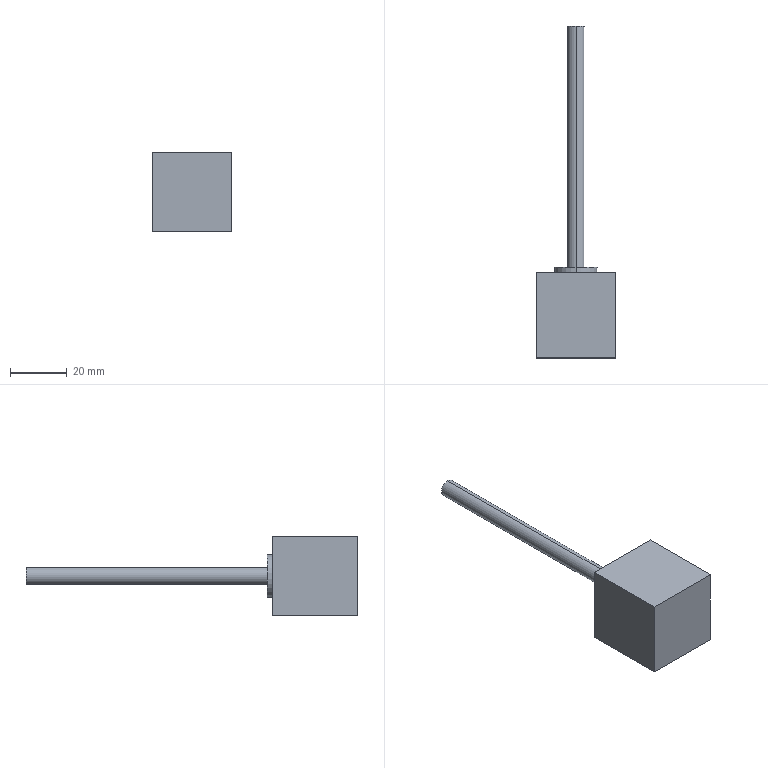Part | SolidWorks | features ICE 3, Extrusion 1, HoleWzd 1 | 1 solid | 28 faces | box 28 x 117 x 28 mm | volume 26125 mm3 | cylinder 12 | cone 8 | plane 8 | commonest cylinder face diameters 2.5 x8 6 x2 15 x2
STEP:
#1=CARTESIAN_POINT('',(-11.5,22.5,10.25));
#2=VERTEX_POINT('',#1);
#3=CARTESIAN_POINT('',(-11.5,22.5,12.75));
#4=VERTEX_POINT('',#3);
#5=CARTESIAN_POINT('',(-11.5,22.5,11.5));
#6=DIRECTION('',(0.,1.,0.));
#7=DIRECTION('',(0.,0.,1.));
#8=AXIS2_PLACEMENT_3D('',#5,#6,#7);
#9=CIRCLE('',#8,1.25);
#10=EDGE_CURVE('',#2,#4,#9,.T.);
#11=ORIENTED_EDGE('',*,*,#10,.F.);
#12=CARTESIAN_POINT('',(-11.5,30.,10.25));
#13=VERTEX_POINT('',#12);
#14=CARTESIAN_POINT('',(-11.5,30.,10.25));
#15=DIRECTION('',(0.,1.,0.));
#16=VECTOR('',#15,1000.);
#17=LINE('',#14,#16);
#18=EDGE_CURVE('',#2,#13,#17,.T.);
#19=ORIENTED_EDGE('',*,*,#18,.T.);
#20=CARTESIAN_POINT('',(-11.5,30.,12.75));
#21=VERTEX_POINT('',#20);
#22=CARTESIAN_POINT('',(-11.5,30.,11.5));
#23=DIRECTION('',(0.,1.,0.));
#24=DIRECTION('',(0.,0.,1.));
#25=AXIS2_PLACEMENT_3D('',#22,#23,#24);
#26=CIRCLE('',#25,1.25);
#27=EDGE_CURVE('',#13,#21,#26,.T.);
#28=ORIENTED_EDGE('',*,*,#27,.T.);
#29=CARTESIAN_POINT('',(-11.5,30.,12.75));
#30=DIRECTION('',(0.,1.,0.));
#31=VECTOR('',#30,1000.);
#32=LINE('',#29,#31);
#33=EDGE_CURVE('',#4,#21,#32,.T.);
#34=ORIENTED_EDGE('',*,*,#33,.F.);
#35=EDGE_LOOP('',(#11,#19,#28,#34));
#36=FACE_OUTER_BOUND('',#35,.T.);
#37=CARTESIAN_POINT('',(-11.5,30.,11.5));
#38=DIRECTION('',(0.,1.,0.));
#39=DIRECTION('',(0.,0.,1.));
#40=AXIS2_PLACEMENT_3D('',#37,#38,#39);
#41=CYLINDRICAL_SURFACE('',#40,1.25);
#42=ADVANCED_FACE('',(#36),#41,.F.);
#43=CARTESIAN_POINT('',(-11.5,21.749,11.5));
#44=VERTEX_POINT('',#43);
#45=CARTESIAN_POINT('',(-11.5,22.5,12.75));
#46=DIRECTION('',(0.,0.515,0.8572));
#47=VECTOR('',#46,1000.);
#48=LINE('',#45,#47);
#49=EDGE_CURVE('',#44,#4,#48,.T.);
#50=ORIENTED_EDGE('',*,*,#49,.F.);
#51=CARTESIAN_POINT('',(-11.5,22.5,10.25));
#52=DIRECTION('',(0.,0.515,-0.8572));
#53=VECTOR('',#52,1000.);
#54=LINE('',#51,#53);
#55=EDGE_CURVE('',#44,#2,#54,.T.);
#56=ORIENTED_EDGE('',*,*,#55,.T.);
#57=ORIENTED_EDGE('',*,*,#10,.T.);
#58=EDGE_LOOP('',(#50,#56,#57));
#59=FACE_OUTER_BOUND('',#58,.T.);
#60=CARTESIAN_POINT('',(-11.5,22.5,11.5));
#61=DIRECTION('',(0.,1.,0.));
#62=DIRECTION('',(0.,0.,1.));
#63=AXIS2_PLACEMENT_3D('',#60,#61,#62);
#64=CONICAL_SURFACE('',#63,1.25,1.03);
#65=ADVANCED_FACE('',(#59),#64,.F.);
#66=CARTESIAN_POINT('',(11.5,22.5,10.25));
#67=VERTEX_POINT('',#66);
#68=CARTESIAN_POINT('',(11.5,22.5,12.75));
#69=VERTEX_POINT('',#68);
#70=CARTESIAN_POINT('',(11.5,22.5,11.5));
#71=DIRECTION('',(0.,1.,0.));
#72=DIRECTION('',(0.,0.,1.));
#73=AXIS2_PLACEMENT_3D('',#70,#71,#72);
#74=CIRCLE('',#73,1.25);
#75=EDGE_CURVE('',#67,#69,#74,.T.);
#76=ORIENTED_EDGE('',*,*,#75,.F.);
#77=CARTESIAN_POINT('',(11.5,30.,10.25));
#78=VERTEX_POINT('',#77);
#79=CARTESIAN_POINT('',(11.5,30.,10.25));
#80=DIRECTION('',(0.,1.,0.));
#81=VECTOR('',#80,1000.);
#82=LINE('',#79,#81);
#83=EDGE_CURVE('',#67,#78,#82,.T.);
#84=ORIENTED_EDGE('',*,*,#83,.T.);
#85=CARTESIAN_POINT('',(11.5,30.,12.75));
#86=VERTEX_POINT('',#85);
#87=CARTESIAN_POINT('',(11.5,30.,11.5));
#88=DIRECTION('',(0.,1.,0.));
#89=DIRECTION('',(0.,0.,1.));
#90=AXIS2_PLACEMENT_3D('',#87,#88,#89);
#91=CIRCLE('',#90,1.25);
#92=EDGE_CURVE('',#78,#86,#91,.T.);
#93=ORIENTED_EDGE('',*,*,#92,.T.);
#94=CARTESIAN_POINT('',(11.5,30.,12.75));
#95=DIRECTION('',(0.,1.,0.));
#96=VECTOR('',#95,1000.);
#97=LINE('',#94,#96);
#98=EDGE_CURVE('',#69,#86,#97,.T.);
#99=ORIENTED_EDGE('',*,*,#98,.F.);
#100=EDGE_LOOP('',(#76,#84,#93,#99));
#101=FACE_OUTER_BOUND('',#100,.T.);
#102=CARTESIAN_POINT('',(11.5,30.,11.5));
#103=DIRECTION('',(0.,1.,0.));
#104=DIRECTION('',(0.,0.,1.));
#105=AXIS2_PLACEMENT_3D('',#102,#103,#104);
#106=CYLINDRICAL_SURFACE('',#105,1.25);
#107=ADVANCED_FACE('',(#101),#106,.F.);
#108=CARTESIAN_POINT('',(11.5,21.749,11.5));
#109=VERTEX_POINT('',#108);
#110=CARTESIAN_POINT('',(11.5,22.5,12.75));
#111=DIRECTION('',(0.,0.515,0.8572));
#112=VECTOR('',#111,1000.);
#113=LINE('',#110,#112);
#114=EDGE_CURVE('',#109,#69,#113,.T.);
#115=ORIENTED_EDGE('',*,*,#114,.F.);
#116=CARTESIAN_POINT('',(11.5,22.5,10.25));
#117=DIRECTION('',(0.,0.515,-0.8572));
#118=VECTOR('',#117,1000.);
#119=LINE('',#116,#118);
#120=EDGE_CURVE('',#109,#67,#119,.T.);
#121=ORIENTED_EDGE('',*,*,#120,.T.);
#122=ORIENTED_EDGE('',*,*,#75,.T.);
#123=EDGE_LOOP('',(#115,#121,#122));
#124=FACE_OUTER_BOUND('',#123,.T.);
#125=CARTESIAN_POINT('',(11.5,22.5,11.5));
#126=DIRECTION('',(0.,1.,0.));
#127=DIRECTION('',(0.,0.,1.));
#128=AXIS2_PLACEMENT_3D('',#125,#126,#127);
#129=CONICAL_SURFACE('',#128,1.25,1.03);
#130=ADVANCED_FACE('',(#124),#129,.F.);
#131=CARTESIAN_POINT('',(-11.5,22.5,-12.75));
#132=VERTEX_POINT('',#131);
#133=CARTESIAN_POINT('',(-11.5,22.5,-10.25));
#134=VERTEX_POINT('',#133);
#135=CARTESIAN_POINT('',(-11.5,22.5,-11.5));
#136=DIRECTION('',(0.,1.,0.));
#137=DIRECTION('',(0.,0.,1.));
#138=AXIS2_PLACEMENT_3D('',#135,#136,#137);
#139=CIRCLE('',#138,1.25);
#140=EDGE_CURVE('',#132,#134,#139,.T.);
#141=ORIENTED_EDGE('',*,*,#140,.F.);
#142=CARTESIAN_POINT('',(-11.5,30.,-12.75));
#143=VERTEX_POINT('',#142);
#144=CARTESIAN_POINT('',(-11.5,30.,-12.75));
#145=DIRECTION('',(0.,1.,0.));
#146=VECTOR('',#145,1000.);
#147=LINE('',#144,#146);
#148=EDGE_CURVE('',#132,#143,#147,.T.);
#149=ORIENTED_EDGE('',*,*,#148,.T.);
#150=CARTESIAN_POINT('',(-11.5,30.,-10.25));
#151=VERTEX_POINT('',#150);
#152=CARTESIAN_POINT('',(-11.5,30.,-11.5));
#153=DIRECTION('',(0.,1.,0.));
#154=DIRECTION('',(0.,0.,1.));
#155=AXIS2_PLACEMENT_3D('',#152,#153,#154);
#156=CIRCLE('',#155,1.25);
#157=EDGE_CURVE('',#143,#151,#156,.T.);
#158=ORIENTED_EDGE('',*,*,#157,.T.);
#159=CARTESIAN_POINT('',(-11.5,30.,-10.25));
#160=DIRECTION('',(0.,1.,0.));
#161=VECTOR('',#160,1000.);
#162=LINE('',#159,#161);
#163=EDGE_CURVE('',#134,#151,#162,.T.);
#164=ORIENTED_EDGE('',*,*,#163,.F.);
#165=EDGE_LOOP('',(#141,#149,#158,#164));
#166=FACE_OUTER_BOUND('',#165,.T.);
#167=CARTESIAN_POINT('',(-11.5,30.,-11.5));
#168=DIRECTION('',(0.,1.,0.));
#169=DIRECTION('',(0.,0.,1.));
#170=AXIS2_PLACEMENT_3D('',#167,#168,#169);
#171=CYLINDRICAL_SURFACE('',#170,1.25);
#172=ADVANCED_FACE('',(#166),#171,.F.);
#173=CARTESIAN_POINT('',(-11.5,21.749,-11.5));
#174=VERTEX_POINT('',#173);
#175=CARTESIAN_POINT('',(-11.5,22.5,-10.25));
#176=DIRECTION('',(0.,0.515,0.8572));
#177=VECTOR('',#176,1000.);
#178=LINE('',#175,#177);
#179=EDGE_CURVE('',#174,#134,#178,.T.);
#180=ORIENTED_EDGE('',*,*,#179,.F.);
#181=CARTESIAN_POINT('',(-11.5,22.5,-12.75));
#182=DIRECTION('',(0.,0.515,-0.8572));
#183=VECTOR('',#182,1000.);
#184=LINE('',#181,#183);
#185=EDGE_CURVE('',#174,#132,#184,.T.);
#186=ORIENTED_EDGE('',*,*,#185,.T.);
#187=ORIENTED_EDGE('',*,*,#140,.T.);
#188=EDGE_LOOP('',(#180,#186,#187));
#189=FACE_OUTER_BOUND('',#188,.T.);
#190=CARTESIAN_POINT('',(-11.5,22.5,-11.5));
#191=DIRECTION('',(0.,1.,0.));
#192=DIRECTION('',(0.,0.,1.));
#193=AXIS2_PLACEMENT_3D('',#190,#191,#192);
#194=CONICAL_SURFACE('',#193,1.25,1.03);
#195=ADVANCED_FACE('',(#189),#194,.F.);
#196=CARTESIAN_POINT('',(11.5,22.5,-12.75));
#197=VERTEX_POINT('',#196);
#198=CARTESIAN_POINT('',(11.5,22.5,-10.25));
#199=VERTEX_POINT('',#198);
#200=CARTESIAN_POINT('',(11.5,22.5,-11.5));
#201=DIRECTION('',(0.,1.,0.));
#202=DIRECTION('',(0.,0.,1.));
#203=AXIS2_PLACEMENT_3D('',#200,#201,#202);
#204=CIRCLE('',#203,1.25);
#205=EDGE_CURVE('',#197,#199,#204,.T.);
#206=ORIENTED_EDGE('',*,*,#205,.F.);
#207=CARTESIAN_POINT('',(11.5,30.,-12.75));
#208=VERTEX_POINT('',#207);
#209=CARTESIAN_POINT('',(11.5,30.,-12.75));
#210=DIRECTION('',(0.,1.,0.));
#211=VECTOR('',#210,1000.);
#212=LINE('',#209,#211);
#213=EDGE_CURVE('',#197,#208,#212,.T.);
#214=ORIENTED_EDGE('',*,*,#213,.T.);
#215=CARTESIAN_POINT('',(11.5,30.,-10.25));
#216=VERTEX_POINT('',#215);
#217=CARTESIAN_POINT('',(11.5,30.,-11.5));
#218=DIRECTION('',(0.,1.,0.));
#219=DIRECTION('',(0.,0.,1.));
#220=AXIS2_PLACEMENT_3D('',#217,#218,#219);
#221=CIRCLE('',#220,1.25);
#222=EDGE_CURVE('',#208,#216,#221,.T.);
#223=ORIENTED_EDGE('',*,*,#222,.T.);
#224=CARTESIAN_POINT('',(11.5,30.,-10.25));
#225=DIRECTION('',(0.,1.,0.));
#226=VECTOR('',#225,1000.);
#227=LINE('',#224,#226);
#228=EDGE_CURVE('',#199,#216,#227,.T.);
#229=ORIENTED_EDGE('',*,*,#228,.F.);
#230=EDGE_LOOP('',(#206,#214,#223,#229));
#231=FACE_OUTER_BOUND('',#230,.T.);
#232=CARTESIAN_POINT('',(11.5,30.,-11.5));
#233=DIRECTION('',(0.,1.,0.));
#234=DIRECTION('',(0.,0.,1.));
#235=AXIS2_PLACEMENT_3D('',#232,#233,#234);
#236=CYLINDRICAL_SURFACE('',#235,1.25);
#237=ADVANCED_FACE('',(#231),#236,.F.);
#238=CARTESIAN_POINT('',(11.5,21.749,-11.5));
#239=VERTEX_POINT('',#238);
#240=CARTESIAN_POINT('',(11.5,22.5,-10.25));
#241=DIRECTION('',(0.,0.515,0.8572));
#242=VECTOR('',#241,1000.);
#243=LINE('',#240,#242);
#244=EDGE_CURVE('',#239,#199,#243,.T.);
#245=ORIENTED_EDGE('',*,*,#244,.F.);
#246=CARTESIAN_POINT('',(11.5,22.5,-12.75));
#247=DIRECTION('',(0.,0.515,-0.8572));
#248=VECTOR('',#247,1000.);
#249=LINE('',#246,#248);
#250=EDGE_CURVE('',#239,#197,#249,.T.);
#251=ORIENTED_EDGE('',*,*,#250,.T.);
#252=ORIENTED_EDGE('',*,*,#205,.T.);
#253=EDGE_LOOP('',(#245,#251,#252));
#254=FACE_OUTER_BOUND('',#253,.T.);
#255=CARTESIAN_POINT('',(11.5,22.5,-11.5));
#256=DIRECTION('',(0.,1.,0.));
#257=DIRECTION('',(0.,0.,1.));
#258=AXIS2_PLACEMENT_3D('',#255,#256,#257);
#259=CONICAL_SURFACE('',#258,1.25,1.03);
#260=ADVANCED_FACE('',(#254),#259,.F.);
#261=CARTESIAN_POINT('',(0.,117.,3.));
#262=VERTEX_POINT('',#261);
#263=CARTESIAN_POINT('',(0.,117.,-3.));
#264=VERTEX_POINT('',#263);
#265=CARTESIAN_POINT('',(0.,117.,0.));
#266=DIRECTION('',(0.,1.,0.));
#267=DIRECTION('',(0.,0.,1.));
#268=AXIS2_PLACEMENT_3D('',#265,#266,#267);
#269=CIRCLE('',#268,3.);
#270=EDGE_CURVE('',#262,#264,#269,.T.);
#271=ORIENTED_EDGE('',*,*,#270,.F.);
#272=CARTESIAN_POINT('',(0.,32.,3.));
#273=VERTEX_POINT('',#272);
#274=CARTESIAN_POINT('',(0.,117.,3.));
#275=DIRECTION('',(0.,-1.,0.));
#276=VECTOR('',#275,1000.);
#277=LINE('',#274,#276);
#278=EDGE_CURVE('',#262,#273,#277,.T.);
#279=ORIENTED_EDGE('',*,*,#278,.T.);
#280=CARTESIAN_POINT('',(0.,32.,-3.));
#281=VERTEX_POINT('',#280);
#282=CARTESIAN_POINT('',(0.,32.,0.));
#283=DIRECTION('',(0.,1.,0.));
#284=DIRECTION('',(0.,0.,1.));
#285=AXIS2_PLACEMENT_3D('',#282,#283,#284);
#286=CIRCLE('',#285,3.);
#287=EDGE_CURVE('',#273,#281,#286,.T.);
#288=ORIENTED_EDGE('',*,*,#287,.T.);
#289=CARTESIAN_POINT('',(0.,117.,-3.));
#290=DIRECTION('',(0.,-1.,0.));
#291=VECTOR('',#290,1000.);
#292=LINE('',#289,#291);
#293=EDGE_CURVE('',#264,#281,#292,.T.);
#294=ORIENTED_EDGE('',*,*,#293,.F.);
#295=EDGE_LOOP('',(#271,#279,#288,#294));
#296=FACE_OUTER_BOUND('',#295,.T.);
#297=CARTESIAN_POINT('',(0.,117.,0.));
#298=DIRECTION('',(0.,-1.,0.));
#299=DIRECTION('',(0.,0.,-1.));
#300=AXIS2_PLACEMENT_3D('',#297,#298,#299);
#301=CYLINDRICAL_SURFACE('',#300,3.);
#302=ADVANCED_FACE('',(#296),#301,.T.);
#303=CARTESIAN_POINT('',(0.,32.,7.5));
#304=VERTEX_POINT('',#303);
#305=CARTESIAN_POINT('',(0.,32.,-7.5));
#306=VERTEX_POINT('',#305);
#307=CARTESIAN_POINT('',(0.,32.,0.));
#308=DIRECTION('',(0.,1.,0.));
#309=DIRECTION('',(0.,0.,1.));
#310=AXIS2_PLACEMENT_3D('',#307,#308,#309);
#311=CIRCLE('',#310,7.5);
#312=EDGE_CURVE('',#304,#306,#311,.T.);
#313=ORIENTED_EDGE('',*,*,#312,.F.);
#314=CARTESIAN_POINT('',(0.,30.,7.5));
#315=VERTEX_POINT('',#314);
#316=CARTESIAN_POINT('',(0.,32.,7.5));
#317=DIRECTION('',(0.,-1.,0.));
#318=VECTOR('',#317,1000.);
#319=LINE('',#316,#318);
#320=EDGE_CURVE('',#304,#315,#319,.T.);
#321=ORIENTED_EDGE('',*,*,#320,.T.);
#322=CARTESIAN_POINT('',(0.,30.,-7.5));
#323=VERTEX_POINT('',#322);
#324=CARTESIAN_POINT('',(0.,30.,0.));
#325=DIRECTION('',(0.,1.,0.));
#326=DIRECTION('',(0.,0.,1.));
#327=AXIS2_PLACEMENT_3D('',#324,#325,#326);
#328=CIRCLE('',#327,7.5);
#329=EDGE_CURVE('',#315,#323,#328,.T.);
#330=ORIENTED_EDGE('',*,*,#329,.T.);
#331=CARTESIAN_POINT('',(0.,32.,-7.5));
#332=DIRECTION('',(0.,-1.,0.));
#333=VECTOR('',#332,1000.);
#334=LINE('',#331,#333);
#335=EDGE_CURVE('',#306,#323,#334,.T.);
#336=ORIENTED_EDGE('',*,*,#335,.F.);
#337=EDGE_LOOP('',(#313,#321,#330,#336));
#338=FACE_OUTER_BOUND('',#337,.T.);
#339=CARTESIAN_POINT('',(0.,32.,0.));
#340=DIRECTION('',(0.,-1.,0.));
#341=DIRECTION('',(0.,0.,-1.));
#342=AXIS2_PLACEMENT_3D('',#339,#340,#341);
#343=CYLINDRICAL_SURFACE('',#342,7.5);
#344=ADVANCED_FACE('',(#338),#343,.T.);
#345=CARTESIAN_POINT('',(14.,0.,14.));
#346=VERTEX_POINT('',#345);
#347=CARTESIAN_POINT('',(14.,0.,-14.));
#348=VERTEX_POINT('',#347);
#349=CARTESIAN_POINT('',(14.,0.,-14.));
#350=DIRECTION('',(0.,0.,-1.));
#351=VECTOR('',#350,1000.);
#352=LINE('',#349,#351);
#353=EDGE_CURVE('',#346,#348,#352,.T.);
#354=ORIENTED_EDGE('',*,*,#353,.T.);
#355=CARTESIAN_POINT('',(14.,30.,-14.));
#356=VERTEX_POINT('',#355);
#357=CARTESIAN_POINT('',(14.,30.,-14.));
#358=DIRECTION('',(0.,-1.,0.));
#359=VECTOR('',#358,1000.);
#360=LINE('',#357,#359);
#361=EDGE_CURVE('',#356,#348,#360,.T.);
#362=ORIENTED_EDGE('',*,*,#361,.F.);
#363=CARTESIAN_POINT('',(14.,30.,14.));
#364=VERTEX_POINT('',#363);
#365=CARTESIAN_POINT('',(14.,30.,-14.));
#366=DIRECTION('',(0.,0.,-1.));
#367=VECTOR('',#366,1000.);
#368=LINE('',#365,#367);
#369=EDGE_CURVE('',#364,#356,#368,.T.);
#370=ORIENTED_EDGE('',*,*,#369,.F.);
#371=CARTESIAN_POINT('',(14.,30.,14.));
#372=DIRECTION('',(0.,-1.,0.));
#373=VECTOR('',#372,1000.);
#374=LINE('',#371,#373);
#375=EDGE_CURVE('',#364,#346,#374,.T.);
#376=ORIENTED_EDGE('',*,*,#375,.T.);
#377=EDGE_LOOP('',(#354,#362,#370,#376));
#378=FACE_OUTER_BOUND('',#377,.T.);
#379=CARTESIAN_POINT('',(14.,30.,-14.));
#380=DIRECTION('',(-1.,0.,0.));
#381=DIRECTION('',(0.,0.,1.));
#382=AXIS2_PLACEMENT_3D('',#379,#380,#381);
#383=PLANE('',#382);
#384=ADVANCED_FACE('',(#378),#383,.F.);
#385=CARTESIAN_POINT('',(-14.,0.,-14.));
#386=VERTEX_POINT('',#385);
#387=CARTESIAN_POINT('',(-14.,0.,-14.));
#388=DIRECTION('',(-1.,0.,0.));
#389=VECTOR('',#388,1000.);
#390=LINE('',#387,#389);
#391=EDGE_CURVE('',#348,#386,#390,.T.);
#392=ORIENTED_EDGE('',*,*,#391,.T.);
#393=CARTESIAN_POINT('',(-14.,30.,-14.));
#394=VERTEX_POINT('',#393);
#395=CARTESIAN_POINT('',(-14.,30.,-14.));
#396=DIRECTION('',(0.,-1.,0.));
#397=VECTOR('',#396,1000.);
#398=LINE('',#395,#397);
#399=EDGE_CURVE('',#394,#386,#398,.T.);
#400=ORIENTED_EDGE('',*,*,#399,.F.);
#401=CARTESIAN_POINT('',(-14.,30.,-14.));
#402=DIRECTION('',(-1.,0.,0.));
#403=VECTOR('',#402,1000.);
#404=LINE('',#401,#403);
#405=EDGE_CURVE('',#356,#394,#404,.T.);
#406=ORIENTED_EDGE('',*,*,#405,.F.);
#407=ORIENTED_EDGE('',*,*,#361,.T.);
#408=EDGE_LOOP('',(#392,#400,#406,#407));
#409=FACE_OUTER_BOUND('',#408,.T.);
#410=CARTESIAN_POINT('',(-14.,30.,-14.));
#411=DIRECTION('',(0.,0.,1.));
#412=DIRECTION('',(1.,0.,0.));
#413=AXIS2_PLACEMENT_3D('',#410,#411,#412);
#414=PLANE('',#413);
#415=ADVANCED_FACE('',(#409),#414,.F.);
#416=CARTESIAN_POINT('',(-14.,0.,14.));
#417=VERTEX_POINT('',#416);
#418=CARTESIAN_POINT('',(-14.,0.,-14.));
#419=DIRECTION('',(0.,0.,1.));
#420=VECTOR('',#419,1000.);
#421=LINE('',#418,#420);
#422=EDGE_CURVE('',#386,#417,#421,.T.);
#423=ORIENTED_EDGE('',*,*,#422,.T.);
#424=CARTESIAN_POINT('',(-14.,30.,14.));
#425=VERTEX_POINT('',#424);
#426=CARTESIAN_POINT('',(-14.,30.,14.));
#427=DIRECTION('',(0.,-1.,0.));
#428=VECTOR('',#427,1000.);
#429=LINE('',#426,#428);
#430=EDGE_CURVE('',#425,#417,#429,.T.);
#431=ORIENTED_EDGE('',*,*,#430,.F.);
#432=CARTESIAN_POINT('',(-14.,30.,-14.));
#433=DIRECTION('',(0.,0.,1.));
#434=VECTOR('',#433,1000.);
#435=LINE('',#432,#434);
#436=EDGE_CURVE('',#394,#425,#435,.T.);
#437=ORIENTED_EDGE('',*,*,#436,.F.);
#438=ORIENTED_EDGE('',*,*,#399,.T.);
#439=EDGE_LOOP('',(#423,#431,#437,#438));
#440=FACE_OUTER_BOUND('',#439,.T.);
#441=CARTESIAN_POINT('',(-14.,30.,-14.));
#442=DIRECTION('',(1.,0.,0.));
#443=DIRECTION('',(0.,0.,-1.));
#444=AXIS2_PLACEMENT_3D('',#441,#442,#443);
#445=PLANE('',#444);
#446=ADVANCED_FACE('',(#440),#445,.F.);
#447=CARTESIAN_POINT('',(-14.,0.,14.));
#448=DIRECTION('',(1.,0.,0.));
#449=VECTOR('',#448,1000.);
#450=LINE('',#447,#449);
#451=EDGE_CURVE('',#417,#346,#450,.T.);
#452=ORIENTED_EDGE('',*,*,#451,.T.);
#453=ORIENTED_EDGE('',*,*,#375,.F.);
#454=CARTESIAN_POINT('',(-14.,30.,14.));
#455=DIRECTION('',(1.,0.,0.));
#456=VECTOR('',#455,1000.);
#457=LINE('',#454,#456);
#458=EDGE_CURVE('',#425,#364,#457,.T.);
#459=ORIENTED_EDGE('',*,*,#458,.F.);
#460=ORIENTED_EDGE('',*,*,#430,.T.);
#461=EDGE_LOOP('',(#452,#453,#459,#460));
#462=FACE_OUTER_BOUND('',#461,.T.);
#463=CARTESIAN_POINT('',(-14.,30.,14.));
#464=DIRECTION('',(0.,0.,-1.));
#465=DIRECTION('',(-1.,0.,0.));
#466=AXIS2_PLACEMENT_3D('',#463,#464,#465);
#467=PLANE('',#466);
#468=ADVANCED_FACE('',(#462),#467,.F.);
#469=CARTESIAN_POINT('',(-11.5,30.,11.5));
#470=DIRECTION('',(0.,1.,0.));
#471=DIRECTION('',(0.,0.,1.));
#472=AXIS2_PLACEMENT_3D('',#469,#470,#471);
#473=CIRCLE('',#472,1.25);
#474=EDGE_CURVE('',#21,#13,#473,.T.);
#475=ORIENTED_EDGE('',*,*,#474,.F.);
#476=ORIENTED_EDGE('',*,*,#27,.F.);
#477=EDGE_LOOP('',(#475,#476));
#478=FACE_BOUND('',#477,.T.);
#479=CARTESIAN_POINT('',(11.5,30.,11.5));
#480=DIRECTION('',(0.,1.,0.));
#481=DIRECTION('',(0.,0.,1.));
#482=AXIS2_PLACEMENT_3D('',#479,#480,#481);
#483=CIRCLE('',#482,1.25);
#484=EDGE_CURVE('',#86,#78,#483,.T.);
#485=ORIENTED_EDGE('',*,*,#484,.F.);
#486=ORIENTED_EDGE('',*,*,#92,.F.);
#487=EDGE_LOOP('',(#485,#486));
#488=FACE_BOUND('',#487,.T.);
#489=CARTESIAN_POINT('',(-11.5,30.,-11.5));
#490=DIRECTION('',(0.,1.,0.));
#491=DIRECTION('',(0.,0.,1.));
#492=AXIS2_PLACEMENT_3D('',#489,#490,#491);
#493=CIRCLE('',#492,1.25);
#494=EDGE_CURVE('',#151,#143,#493,.T.);
#495=ORIENTED_EDGE('',*,*,#494,.F.);
#496=ORIENTED_EDGE('',*,*,#157,.F.);
#497=EDGE_LOOP('',(#495,#496));
#498=FACE_BOUND('',#497,.T.);
#499=CARTESIAN_POINT('',(11.5,30.,-11.5));
#500=DIRECTION('',(0.,1.,0.));
#501=DIRECTION('',(0.,0.,1.));
#502=AXIS2_PLACEMENT_3D('',#499,#500,#501);
#503=CIRCLE('',#502,1.25);
#504=EDGE_CURVE('',#216,#208,#503,.T.);
#505=ORIENTED_EDGE('',*,*,#504,.F.);
#506=ORIENTED_EDGE('',*,*,#222,.F.);
#507=EDGE_LOOP('',(#505,#506));
#508=FACE_BOUND('',#507,.T.);
#509=CARTESIAN_POINT('',(0.,30.,0.));
#510=DIRECTION('',(0.,1.,0.));
#511=DIRECTION('',(0.,0.,1.));
#512=AXIS2_PLACEMENT_3D('',#509,#510,#511);
#513=CIRCLE('',#512,7.5);
#514=EDGE_CURVE('',#323,#315,#513,.T.);
#515=ORIENTED_EDGE('',*,*,#514,.F.);
#516=ORIENTED_EDGE('',*,*,#329,.F.);
#517=EDGE_LOOP('',(#515,#516));
#518=FACE_BOUND('',#517,.T.);
#519=ORIENTED_EDGE('',*,*,#369,.T.);
#520=ORIENTED_EDGE('',*,*,#405,.T.);
#521=ORIENTED_EDGE('',*,*,#436,.T.);
#522=ORIENTED_EDGE('',*,*,#458,.T.);
#523=EDGE_LOOP('',(#519,#520,#521,#522));
#524=FACE_OUTER_BOUND('',#523,.T.);
#525=CARTESIAN_POINT('',(0.,30.,0.));
#526=DIRECTION('',(0.,1.,0.));
#527=DIRECTION('',(0.,0.,1.));
#528=AXIS2_PLACEMENT_3D('',#525,#526,#527);
#529=PLANE('',#528);
#530=ADVANCED_FACE('',(#478,#488,#498,#508,#518,#524),#529,.T.);
#531=ORIENTED_EDGE('',*,*,#353,.F.);
#532=ORIENTED_EDGE('',*,*,#451,.F.);
#533=ORIENTED_EDGE('',*,*,#422,.F.);
#534=ORIENTED_EDGE('',*,*,#391,.F.);
#535=EDGE_LOOP('',(#531,#532,#533,#534));
#536=FACE_OUTER_BOUND('',#535,.T.);
#537=CARTESIAN_POINT('',(0.,0.,0.));
#538=DIRECTION('',(0.,1.,0.));
#539=DIRECTION('',(0.,0.,1.));
#540=AXIS2_PLACEMENT_3D('',#537,#538,#539);
#541=PLANE('',#540);
#542=ADVANCED_FACE('',(#536),#541,.F.);
#543=ORIENTED_EDGE('',*,*,#320,.F.);
#544=CARTESIAN_POINT('',(0.,32.,0.));
#545=DIRECTION('',(0.,1.,0.));
#546=DIRECTION('',(0.,0.,1.));
#547=AXIS2_PLACEMENT_3D('',#544,#545,#546);
#548=CIRCLE('',#547,7.5);
#549=EDGE_CURVE('',#306,#304,#548,.T.);
#550=ORIENTED_EDGE('',*,*,#549,.F.);
#551=ORIENTED_EDGE('',*,*,#335,.T.);
#552=ORIENTED_EDGE('',*,*,#514,.T.);
#553=EDGE_LOOP('',(#543,#550,#551,#552));
#554=FACE_OUTER_BOUND('',#553,.T.);
#555=CARTESIAN_POINT('',(0.,32.,0.));
#556=DIRECTION('',(0.,-1.,0.));
#557=DIRECTION('',(0.,0.,-1.));
#558=AXIS2_PLACEMENT_3D('',#555,#556,#557);
#559=CYLINDRICAL_SURFACE('',#558,7.5);
#560=ADVANCED_FACE('',(#554),#559,.T.);
#561=CARTESIAN_POINT('',(0.,32.,0.));
#562=DIRECTION('',(0.,1.,0.));
#563=DIRECTION('',(0.,0.,1.));
#564=AXIS2_PLACEMENT_3D('',#561,#562,#563);
#565=CIRCLE('',#564,3.);
#566=EDGE_CURVE('',#281,#273,#565,.T.);
#567=ORIENTED_EDGE('',*,*,#566,.F.);
#568=ORIENTED_EDGE('',*,*,#287,.F.);
#569=EDGE_LOOP('',(#567,#568));
#570=FACE_BOUND('',#569,.T.);
#571=ORIENTED_EDGE('',*,*,#549,.T.);
#572=ORIENTED_EDGE('',*,*,#312,.T.);
#573=EDGE_LOOP('',(#571,#572));
#574=FACE_OUTER_BOUND('',#573,.T.);
#575=CARTESIAN_POINT('',(0.,32.,0.));
#576=DIRECTION('',(0.,1.,0.));
#577=DIRECTION('',(0.,0.,1.));
#578=AXIS2_PLACEMENT_3D('',#575,#576,#577);
#579=PLANE('',#578);
#580=ADVANCED_FACE('',(#570,#574),#579,.T.);
#581=ORIENTED_EDGE('',*,*,#278,.F.);
#582=CARTESIAN_POINT('',(0.,117.,0.));
#583=DIRECTION('',(0.,1.,0.));
#584=DIRECTION('',(0.,0.,1.));
#585=AXIS2_PLACEMENT_3D('',#582,#583,#584);
#586=CIRCLE('',#585,3.);
#587=EDGE_CURVE('',#264,#262,#586,.T.);
#588=ORIENTED_EDGE('',*,*,#587,.F.);
#589=ORIENTED_EDGE('',*,*,#293,.T.);
#590=ORIENTED_EDGE('',*,*,#566,.T.);
#591=EDGE_LOOP('',(#581,#588,#589,#590));
#592=FACE_OUTER_BOUND('',#591,.T.);
#593=CARTESIAN_POINT('',(0.,117.,0.));
#594=DIRECTION('',(0.,-1.,0.));
#595=DIRECTION('',(0.,0.,-1.));
#596=AXIS2_PLACEMENT_3D('',#593,#594,#595);
#597=CYLINDRICAL_SURFACE('',#596,3.);
#598=ADVANCED_FACE('',(#592),#597,.T.);
#599=ORIENTED_EDGE('',*,*,#587,.T.);
#600=ORIENTED_EDGE('',*,*,#270,.T.);
#601=EDGE_LOOP('',(#599,#600));
#602=FACE_OUTER_BOUND('',#601,.T.);
#603=CARTESIAN_POINT('',(0.,117.,0.));
#604=DIRECTION('',(0.,1.,0.));
#605=DIRECTION('',(0.,0.,1.));
#606=AXIS2_PLACEMENT_3D('',#603,#604,#605);
#607=PLANE('',#606);
#608=ADVANCED_FACE('',(#602),#607,.T.);
#609=ORIENTED_EDGE('',*,*,#250,.F.);
#610=ORIENTED_EDGE('',*,*,#244,.T.);
#611=CARTESIAN_POINT('',(11.5,22.5,-11.5));
#612=DIRECTION('',(0.,1.,0.));
#613=DIRECTION('',(0.,0.,1.));
#614=AXIS2_PLACEMENT_3D('',#611,#612,#613);
#615=CIRCLE('',#614,1.25);
#616=EDGE_CURVE('',#199,#197,#615,.T.);
#617=ORIENTED_EDGE('',*,*,#616,.T.);
#618=EDGE_LOOP('',(#609,#610,#617));
#619=FACE_OUTER_BOUND('',#618,.T.);
#620=CARTESIAN_POINT('',(11.5,22.5,-11.5));
#621=DIRECTION('',(0.,1.,0.));
#622=DIRECTION('',(0.,0.,1.));
#623=AXIS2_PLACEMENT_3D('',#620,#621,#622);
#624=CONICAL_SURFACE('',#623,1.25,1.03);
#625=ADVANCED_FACE('',(#619),#624,.F.);
#626=ORIENTED_EDGE('',*,*,#213,.F.);
#627=ORIENTED_EDGE('',*,*,#616,.F.);
#628=ORIENTED_EDGE('',*,*,#228,.T.);
#629=ORIENTED_EDGE('',*,*,#504,.T.);
#630=EDGE_LOOP('',(#626,#627,#628,#629));
#631=FACE_OUTER_BOUND('',#630,.T.);
#632=CARTESIAN_POINT('',(11.5,30.,-11.5));
#633=DIRECTION('',(0.,1.,0.));
#634=DIRECTION('',(0.,0.,1.));
#635=AXIS2_PLACEMENT_3D('',#632,#633,#634);
#636=CYLINDRICAL_SURFACE('',#635,1.25);
#637=ADVANCED_FACE('',(#631),#636,.F.);
#638=ORIENTED_EDGE('',*,*,#185,.F.);
#639=ORIENTED_EDGE('',*,*,#179,.T.);
#640=CARTESIAN_POINT('',(-11.5,22.5,-11.5));
#641=DIRECTION('',(0.,1.,0.));
#642=DIRECTION('',(0.,0.,1.));
#643=AXIS2_PLACEMENT_3D('',#640,#641,#642);
#644=CIRCLE('',#643,1.25);
#645=EDGE_CURVE('',#134,#132,#644,.T.);
#646=ORIENTED_EDGE('',*,*,#645,.T.);
#647=EDGE_LOOP('',(#638,#639,#646));
#648=FACE_OUTER_BOUND('',#647,.T.);
#649=CARTESIAN_POINT('',(-11.5,22.5,-11.5));
#650=DIRECTION('',(0.,1.,0.));
#651=DIRECTION('',(0.,0.,1.));
#652=AXIS2_PLACEMENT_3D('',#649,#650,#651);
#653=CONICAL_SURFACE('',#652,1.25,1.03);
#654=ADVANCED_FACE('',(#648),#653,.F.);
#655=ORIENTED_EDGE('',*,*,#148,.F.);
#656=ORIENTED_EDGE('',*,*,#645,.F.);
#657=ORIENTED_EDGE('',*,*,#163,.T.);
#658=ORIENTED_EDGE('',*,*,#494,.T.);
#659=EDGE_LOOP('',(#655,#656,#657,#658));
#660=FACE_OUTER_BOUND('',#659,.T.);
#661=CARTESIAN_POINT('',(-11.5,30.,-11.5));
#662=DIRECTION('',(0.,1.,0.));
#663=DIRECTION('',(0.,0.,1.));
#664=AXIS2_PLACEMENT_3D('',#661,#662,#663);
#665=CYLINDRICAL_SURFACE('',#664,1.25);
#666=ADVANCED_FACE('',(#660),#665,.F.);
#667=ORIENTED_EDGE('',*,*,#120,.F.);
#668=ORIENTED_EDGE('',*,*,#114,.T.);
#669=CARTESIAN_POINT('',(11.5,22.5,11.5));
#670=DIRECTION('',(0.,1.,0.));
#671=DIRECTION('',(0.,0.,1.));
#672=AXIS2_PLACEMENT_3D('',#669,#670,#671);
#673=CIRCLE('',#672,1.25);
#674=EDGE_CURVE('',#69,#67,#673,.T.);
#675=ORIENTED_EDGE('',*,*,#674,.T.);
#676=EDGE_LOOP('',(#667,#668,#675));
#677=FACE_OUTER_BOUND('',#676,.T.);
#678=CARTESIAN_POINT('',(11.5,22.5,11.5));
#679=DIRECTION('',(0.,1.,0.));
#680=DIRECTION('',(0.,0.,1.));
#681=AXIS2_PLACEMENT_3D('',#678,#679,#680);
#682=CONICAL_SURFACE('',#681,1.25,1.03);
#683=ADVANCED_FACE('',(#677),#682,.F.);
#684=ORIENTED_EDGE('',*,*,#83,.F.);
#685=ORIENTED_EDGE('',*,*,#674,.F.);
#686=ORIENTED_EDGE('',*,*,#98,.T.);
#687=ORIENTED_EDGE('',*,*,#484,.T.);
#688=EDGE_LOOP('',(#684,#685,#686,#687));
#689=FACE_OUTER_BOUND('',#688,.T.);
#690=CARTESIAN_POINT('',(11.5,30.,11.5));
#691=DIRECTION('',(0.,1.,0.));
#692=DIRECTION('',(0.,0.,1.));
#693=AXIS2_PLACEMENT_3D('',#690,#691,#692);
#694=CYLINDRICAL_SURFACE('',#693,1.25);
#695=ADVANCED_FACE('',(#689),#694,.F.);
#696=ORIENTED_EDGE('',*,*,#55,.F.);
#697=ORIENTED_EDGE('',*,*,#49,.T.);
#698=CARTESIAN_POINT('',(-11.5,22.5,11.5));
#699=DIRECTION('',(0.,1.,0.));
#700=DIRECTION('',(0.,0.,1.));
#701=AXIS2_PLACEMENT_3D('',#698,#699,#700);
#702=CIRCLE('',#701,1.25);
#703=EDGE_CURVE('',#4,#2,#702,.T.);
#704=ORIENTED_EDGE('',*,*,#703,.T.);
#705=EDGE_LOOP('',(#696,#697,#704));
#706=FACE_OUTER_BOUND('',#705,.T.);
#707=CARTESIAN_POINT('',(-11.5,22.5,11.5));
#708=DIRECTION('',(0.,1.,0.));
#709=DIRECTION('',(0.,0.,1.));
#710=AXIS2_PLACEMENT_3D('',#707,#708,#709);
#711=CONICAL_SURFACE('',#710,1.25,1.03);
#712=ADVANCED_FACE('',(#706),#711,.F.);
#713=ORIENTED_EDGE('',*,*,#18,.F.);
#714=ORIENTED_EDGE('',*,*,#703,.F.);
#715=ORIENTED_EDGE('',*,*,#33,.T.);
#716=ORIENTED_EDGE('',*,*,#474,.T.);
#717=EDGE_LOOP('',(#713,#714,#715,#716));
#718=FACE_OUTER_BOUND('',#717,.T.);
#719=CARTESIAN_POINT('',(-11.5,30.,11.5));
#720=DIRECTION('',(0.,1.,0.));
#721=DIRECTION('',(0.,0.,1.));
#722=AXIS2_PLACEMENT_3D('',#719,#720,#721);
#723=CYLINDRICAL_SURFACE('',#722,1.25);
#724=ADVANCED_FACE('',(#718),#723,.F.);
#725=CLOSED_SHELL('',(#42,#65,#107,#130,#172,#195,#237,#260,#302,#344,#384,#415,#446,#468,#530,#542,#560,#580,#598,#608,#625,#637,#654,#666,#683,#695,#712,#724));
#726=MANIFOLD_SOLID_BREP('',#725);
#727=CARTESIAN_POINT('',(0.,0.,0.));
#728=DIRECTION('',(0.,0.,1.));
#729=DIRECTION('',(1.,0.,0.));
#730=AXIS2_PLACEMENT_3D('',#727,#728,#729);
#731=(LENGTH_UNIT()NAMED_UNIT(*)SI_UNIT(.MILLI.,.METRE.));
#732=UNCERTAINTY_MEASURE_WITH_UNIT(LENGTH_MEASURE(0.00001),#731,'','');
#733=(NAMED_UNIT(*)PLANE_ANGLE_UNIT()SI_UNIT($,.RADIAN.));
#734=(NAMED_UNIT(*)SI_UNIT($,.STERADIAN.)SOLID_ANGLE_UNIT());
#735=(GEOMETRIC_REPRESENTATION_CONTEXT(3)GLOBAL_UNCERTAINTY_ASSIGNED_CONTEXT((#732))GLOBAL_UNIT_ASSIGNED_CONTEXT((#731,#733,#734))REPRESENTATION_CONTEXT('',''));
#736=ADVANCED_BREP_SHAPE_REPRESENTATION('',(#726,#730),#735);